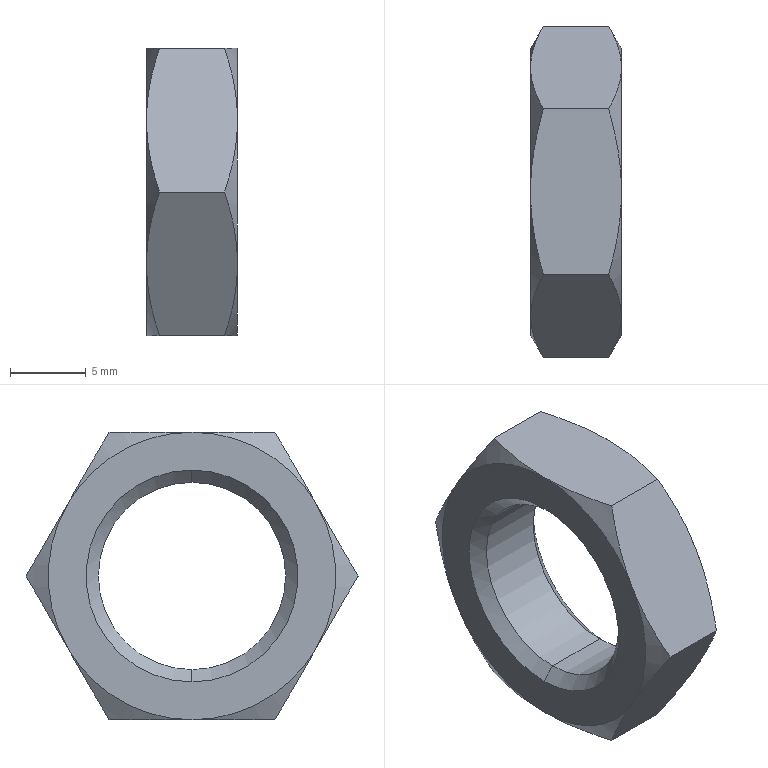Part | SolidWorks | features BaseBody 1 | 1 solid | 26 faces | box 6 x 21.939 x 19 mm | volume 1112 mm3 | cone 16 | plane 8 | cylinder 2 | commonest cylinder face diameters 12.376 x2
STEP:
#1=CARTESIAN_POINT('',(5.188,0.,-6.188));
#2=VERTEX_POINT('',#1);
#3=CARTESIAN_POINT('',(5.188,-6.188,0.));
#4=VERTEX_POINT('',#3);
#5=CARTESIAN_POINT('',(5.188,0.,0.));
#6=DIRECTION('',(-1.,0.,0.));
#7=DIRECTION('',(0.,0.,1.));
#8=AXIS2_PLACEMENT_3D('',#5,#6,#7);
#9=CIRCLE('',#8,6.188);
#10=EDGE_CURVE('',#2,#4,#9,.T.);
#11=ORIENTED_EDGE('',*,*,#10,.F.);
#12=CARTESIAN_POINT('',(0.812,0.,-6.188));
#13=VERTEX_POINT('',#12);
#14=CARTESIAN_POINT('',(50.,0.,-6.188));
#15=DIRECTION('',(-1.,0.,0.));
#16=VECTOR('',#15,1000.);
#17=LINE('',#14,#16);
#18=EDGE_CURVE('',#2,#13,#17,.T.);
#19=ORIENTED_EDGE('',*,*,#18,.T.);
#20=CARTESIAN_POINT('',(0.812,0.,6.188));
#21=VERTEX_POINT('',#20);
#22=CARTESIAN_POINT('',(0.812,0.,0.));
#23=DIRECTION('',(1.,0.,0.));
#24=DIRECTION('',(0.,0.,1.));
#25=AXIS2_PLACEMENT_3D('',#22,#23,#24);
#26=CIRCLE('',#25,6.188);
#27=EDGE_CURVE('',#21,#13,#26,.T.);
#28=ORIENTED_EDGE('',*,*,#27,.F.);
#29=CARTESIAN_POINT('',(5.188,0.,6.188));
#30=VERTEX_POINT('',#29);
#31=CARTESIAN_POINT('',(50.,0.,6.188));
#32=DIRECTION('',(-1.,0.,0.));
#33=VECTOR('',#32,1000.);
#34=LINE('',#31,#33);
#35=EDGE_CURVE('',#30,#21,#34,.T.);
#36=ORIENTED_EDGE('',*,*,#35,.F.);
#37=CARTESIAN_POINT('',(5.188,0.,0.));
#38=DIRECTION('',(-1.,0.,0.));
#39=DIRECTION('',(0.,0.,1.));
#40=AXIS2_PLACEMENT_3D('',#37,#38,#39);
#41=CIRCLE('',#40,6.188);
#42=EDGE_CURVE('',#4,#30,#41,.T.);
#43=ORIENTED_EDGE('',*,*,#42,.F.);
#44=EDGE_LOOP('',(#11,#19,#28,#36,#43));
#45=FACE_OUTER_BOUND('',#44,.T.);
#46=CARTESIAN_POINT('',(50.,0.,0.));
#47=DIRECTION('',(-1.,0.,0.));
#48=DIRECTION('',(0.,0.,1.));
#49=AXIS2_PLACEMENT_3D('',#46,#47,#48);
#50=CYLINDRICAL_SURFACE('',#49,6.188);
#51=ADVANCED_FACE('',(#45),#50,.F.);
#52=ORIENTED_EDGE('',*,*,#27,.T.);
#53=CARTESIAN_POINT('',(0.,0.,-7.));
#54=VERTEX_POINT('',#53);
#55=CARTESIAN_POINT('',(0.,0.,-7.));
#56=DIRECTION('',(-0.7071,0.,-0.7071));
#57=VECTOR('',#56,1000.);
#58=LINE('',#55,#57);
#59=EDGE_CURVE('',#13,#54,#58,.T.);
#60=ORIENTED_EDGE('',*,*,#59,.T.);
#61=CARTESIAN_POINT('',(0.,0.,7.));
#62=VERTEX_POINT('',#61);
#63=CARTESIAN_POINT('',(0.,0.,0.));
#64=DIRECTION('',(1.,0.,0.));
#65=DIRECTION('',(0.,0.,1.));
#66=AXIS2_PLACEMENT_3D('',#63,#64,#65);
#67=CIRCLE('',#66,7.);
#68=EDGE_CURVE('',#62,#54,#67,.T.);
#69=ORIENTED_EDGE('',*,*,#68,.F.);
#70=CARTESIAN_POINT('',(0.,0.,7.));
#71=DIRECTION('',(-0.7071,0.,0.7071));
#72=VECTOR('',#71,1000.);
#73=LINE('',#70,#72);
#74=EDGE_CURVE('',#21,#62,#73,.T.);
#75=ORIENTED_EDGE('',*,*,#74,.F.);
#76=EDGE_LOOP('',(#52,#60,#69,#75));
#77=FACE_OUTER_BOUND('',#76,.T.);
#78=CARTESIAN_POINT('',(0.,0.,0.));
#79=DIRECTION('',(-1.,0.,0.));
#80=DIRECTION('',(0.,0.,1.));
#81=AXIS2_PLACEMENT_3D('',#78,#79,#80);
#82=CONICAL_SURFACE('',#81,7.,0.7854);
#83=ADVANCED_FACE('',(#77),#82,.F.);
#84=CARTESIAN_POINT('',(5.188,6.188,0.));
#85=VERTEX_POINT('',#84);
#86=CARTESIAN_POINT('',(5.188,0.,0.));
#87=DIRECTION('',(-1.,0.,0.));
#88=DIRECTION('',(0.,0.,1.));
#89=AXIS2_PLACEMENT_3D('',#86,#87,#88);
#90=CIRCLE('',#89,6.188);
#91=EDGE_CURVE('',#85,#2,#90,.T.);
#92=ORIENTED_EDGE('',*,*,#91,.T.);
#93=ORIENTED_EDGE('',*,*,#10,.T.);
#94=CARTESIAN_POINT('',(6.,-7.,0.));
#95=VERTEX_POINT('',#94);
#96=CARTESIAN_POINT('',(6.,-7.,0.));
#97=DIRECTION('',(0.7071,-0.7071,0.));
#98=VECTOR('',#97,1000.);
#99=LINE('',#96,#98);
#100=EDGE_CURVE('',#4,#95,#99,.T.);
#101=ORIENTED_EDGE('',*,*,#100,.T.);
#102=CARTESIAN_POINT('',(6.,7.,0.));
#103=VERTEX_POINT('',#102);
#104=CARTESIAN_POINT('',(6.,0.,0.));
#105=DIRECTION('',(-1.,0.,0.));
#106=DIRECTION('',(0.,1.,0.));
#107=AXIS2_PLACEMENT_3D('',#104,#105,#106);
#108=CIRCLE('',#107,7.);
#109=EDGE_CURVE('',#103,#95,#108,.T.);
#110=ORIENTED_EDGE('',*,*,#109,.F.);
#111=CARTESIAN_POINT('',(6.,7.,0.));
#112=DIRECTION('',(0.7071,0.7071,0.));
#113=VECTOR('',#112,1000.);
#114=LINE('',#111,#113);
#115=EDGE_CURVE('',#85,#103,#114,.T.);
#116=ORIENTED_EDGE('',*,*,#115,.F.);
#117=EDGE_LOOP('',(#92,#93,#101,#110,#116));
#118=FACE_OUTER_BOUND('',#117,.T.);
#119=CARTESIAN_POINT('',(6.,0.,0.));
#120=DIRECTION('',(1.,0.,0.));
#121=DIRECTION('',(0.,1.,0.));
#122=AXIS2_PLACEMENT_3D('',#119,#120,#121);
#123=CONICAL_SURFACE('',#122,7.,0.7854);
#124=ADVANCED_FACE('',(#118),#123,.F.);
#125=ORIENTED_EDGE('',*,*,#18,.F.);
#126=ORIENTED_EDGE('',*,*,#91,.F.);
#127=CARTESIAN_POINT('',(5.188,0.,0.));
#128=DIRECTION('',(-1.,0.,0.));
#129=DIRECTION('',(0.,0.,1.));
#130=AXIS2_PLACEMENT_3D('',#127,#128,#129);
#131=CIRCLE('',#130,6.188);
#132=EDGE_CURVE('',#30,#85,#131,.T.);
#133=ORIENTED_EDGE('',*,*,#132,.F.);
#134=ORIENTED_EDGE('',*,*,#35,.T.);
#135=CARTESIAN_POINT('',(0.812,0.,0.));
#136=DIRECTION('',(1.,0.,0.));
#137=DIRECTION('',(0.,0.,1.));
#138=AXIS2_PLACEMENT_3D('',#135,#136,#137);
#139=CIRCLE('',#138,6.188);
#140=EDGE_CURVE('',#13,#21,#139,.T.);
#141=ORIENTED_EDGE('',*,*,#140,.F.);
#142=EDGE_LOOP('',(#125,#126,#133,#134,#141));
#143=FACE_OUTER_BOUND('',#142,.T.);
#144=CARTESIAN_POINT('',(50.,0.,0.));
#145=DIRECTION('',(-1.,0.,0.));
#146=DIRECTION('',(0.,0.,1.));
#147=AXIS2_PLACEMENT_3D('',#144,#145,#146);
#148=CYLINDRICAL_SURFACE('',#147,6.188);
#149=ADVANCED_FACE('',(#143),#148,.F.);
#150=ORIENTED_EDGE('',*,*,#59,.F.);
#151=ORIENTED_EDGE('',*,*,#140,.T.);
#152=ORIENTED_EDGE('',*,*,#74,.T.);
#153=CARTESIAN_POINT('',(0.,0.,0.));
#154=DIRECTION('',(1.,0.,0.));
#155=DIRECTION('',(0.,0.,1.));
#156=AXIS2_PLACEMENT_3D('',#153,#154,#155);
#157=CIRCLE('',#156,7.);
#158=EDGE_CURVE('',#54,#62,#157,.T.);
#159=ORIENTED_EDGE('',*,*,#158,.F.);
#160=EDGE_LOOP('',(#150,#151,#152,#159));
#161=FACE_OUTER_BOUND('',#160,.T.);
#162=CARTESIAN_POINT('',(0.,0.,0.));
#163=DIRECTION('',(-1.,0.,0.));
#164=DIRECTION('',(0.,0.,1.));
#165=AXIS2_PLACEMENT_3D('',#162,#163,#164);
#166=CONICAL_SURFACE('',#165,7.,0.7854);
#167=ADVANCED_FACE('',(#161),#166,.F.);
#168=ORIENTED_EDGE('',*,*,#100,.F.);
#169=ORIENTED_EDGE('',*,*,#42,.T.);
#170=ORIENTED_EDGE('',*,*,#132,.T.);
#171=ORIENTED_EDGE('',*,*,#115,.T.);
#172=CARTESIAN_POINT('',(6.,0.,0.));
#173=DIRECTION('',(-1.,0.,0.));
#174=DIRECTION('',(0.,1.,0.));
#175=AXIS2_PLACEMENT_3D('',#172,#173,#174);
#176=CIRCLE('',#175,7.);
#177=EDGE_CURVE('',#95,#103,#176,.T.);
#178=ORIENTED_EDGE('',*,*,#177,.F.);
#179=EDGE_LOOP('',(#168,#169,#170,#171,#178));
#180=FACE_OUTER_BOUND('',#179,.T.);
#181=CARTESIAN_POINT('',(6.,0.,0.));
#182=DIRECTION('',(1.,0.,0.));
#183=DIRECTION('',(0.,1.,0.));
#184=AXIS2_PLACEMENT_3D('',#181,#182,#183);
#185=CONICAL_SURFACE('',#184,7.,0.7854);
#186=ADVANCED_FACE('',(#180),#185,.F.);
#187=CARTESIAN_POINT('',(0.,-8.227,4.75));
#188=VERTEX_POINT('',#187);
#189=CARTESIAN_POINT('',(0.,0.,9.5));
#190=VERTEX_POINT('',#189);
#191=CARTESIAN_POINT('',(0.,0.,0.));
#192=DIRECTION('',(-1.,0.,0.));
#193=DIRECTION('',(0.,1.,0.));
#194=AXIS2_PLACEMENT_3D('',#191,#192,#193);
#195=CIRCLE('',#194,9.5);
#196=EDGE_CURVE('',#188,#190,#195,.T.);
#197=ORIENTED_EDGE('',*,*,#196,.T.);
#198=CARTESIAN_POINT('',(0.,8.227,4.75));
#199=VERTEX_POINT('',#198);
#200=CARTESIAN_POINT('',(0.,0.,0.));
#201=DIRECTION('',(-1.,0.,0.));
#202=DIRECTION('',(0.,1.,0.));
#203=AXIS2_PLACEMENT_3D('',#200,#201,#202);
#204=CIRCLE('',#203,9.5);
#205=EDGE_CURVE('',#190,#199,#204,.T.);
#206=ORIENTED_EDGE('',*,*,#205,.T.);
#207=CARTESIAN_POINT('',(0.,8.227,-4.75));
#208=VERTEX_POINT('',#207);
#209=CARTESIAN_POINT('',(0.,0.,0.));
#210=DIRECTION('',(-1.,0.,0.));
#211=DIRECTION('',(0.,0.,-1.));
#212=AXIS2_PLACEMENT_3D('',#209,#210,#211);
#213=CIRCLE('',#212,9.5);
#214=EDGE_CURVE('',#199,#208,#213,.T.);
#215=ORIENTED_EDGE('',*,*,#214,.T.);
#216=CARTESIAN_POINT('',(0.,0.,-9.5));
#217=VERTEX_POINT('',#216);
#218=CARTESIAN_POINT('',(0.,0.,0.));
#219=DIRECTION('',(-1.,0.,0.));
#220=DIRECTION('',(0.,1.,0.));
#221=AXIS2_PLACEMENT_3D('',#218,#219,#220);
#222=CIRCLE('',#221,9.5);
#223=EDGE_CURVE('',#208,#217,#222,.T.);
#224=ORIENTED_EDGE('',*,*,#223,.T.);
#225=CARTESIAN_POINT('',(0.,-8.227,-4.75));
#226=VERTEX_POINT('',#225);
#227=CARTESIAN_POINT('',(0.,0.,0.));
#228=DIRECTION('',(-1.,0.,0.));
#229=DIRECTION('',(0.,1.,0.));
#230=AXIS2_PLACEMENT_3D('',#227,#228,#229);
#231=CIRCLE('',#230,9.5);
#232=EDGE_CURVE('',#217,#226,#231,.T.);
#233=ORIENTED_EDGE('',*,*,#232,.T.);
#234=CARTESIAN_POINT('',(0.,0.,0.));
#235=DIRECTION('',(-1.,0.,0.));
#236=DIRECTION('',(0.,0.,-1.));
#237=AXIS2_PLACEMENT_3D('',#234,#235,#236);
#238=CIRCLE('',#237,9.5);
#239=EDGE_CURVE('',#226,#188,#238,.T.);
#240=ORIENTED_EDGE('',*,*,#239,.T.);
#241=EDGE_LOOP('',(#197,#206,#215,#224,#233,#240));
#242=FACE_OUTER_BOUND('',#241,.T.);
#243=ORIENTED_EDGE('',*,*,#68,.T.);
#244=ORIENTED_EDGE('',*,*,#158,.T.);
#245=EDGE_LOOP('',(#243,#244));
#246=FACE_BOUND('',#245,.T.);
#247=CARTESIAN_POINT('',(0.,9.5,0.));
#248=DIRECTION('',(-1.,0.,0.));
#249=DIRECTION('',(0.,0.,1.));
#250=AXIS2_PLACEMENT_3D('',#247,#248,#249);
#251=PLANE('',#250);
#252=ADVANCED_FACE('',(#242,#246),#251,.T.);
#253=ORIENTED_EDGE('',*,*,#109,.T.);
#254=ORIENTED_EDGE('',*,*,#177,.T.);
#255=EDGE_LOOP('',(#253,#254));
#256=FACE_BOUND('',#255,.T.);
#257=CARTESIAN_POINT('',(6.,-8.227,4.75));
#258=VERTEX_POINT('',#257);
#259=CARTESIAN_POINT('',(6.,-8.227,-4.75));
#260=VERTEX_POINT('',#259);
#261=CARTESIAN_POINT('',(6.,0.,0.));
#262=DIRECTION('',(1.,0.,0.));
#263=DIRECTION('',(0.,0.,1.));
#264=AXIS2_PLACEMENT_3D('',#261,#262,#263);
#265=CIRCLE('',#264,9.5);
#266=EDGE_CURVE('',#258,#260,#265,.T.);
#267=ORIENTED_EDGE('',*,*,#266,.T.);
#268=CARTESIAN_POINT('',(6.,0.,-9.5));
#269=VERTEX_POINT('',#268);
#270=CARTESIAN_POINT('',(6.,0.,0.));
#271=DIRECTION('',(1.,0.,0.));
#272=DIRECTION('',(0.,0.,1.));
#273=AXIS2_PLACEMENT_3D('',#270,#271,#272);
#274=CIRCLE('',#273,9.5);
#275=EDGE_CURVE('',#260,#269,#274,.T.);
#276=ORIENTED_EDGE('',*,*,#275,.T.);
#277=CARTESIAN_POINT('',(6.,8.227,-4.75));
#278=VERTEX_POINT('',#277);
#279=CARTESIAN_POINT('',(6.,0.,0.));
#280=DIRECTION('',(1.,0.,0.));
#281=DIRECTION('',(0.,0.,1.));
#282=AXIS2_PLACEMENT_3D('',#279,#280,#281);
#283=CIRCLE('',#282,9.5);
#284=EDGE_CURVE('',#269,#278,#283,.T.);
#285=ORIENTED_EDGE('',*,*,#284,.T.);
#286=CARTESIAN_POINT('',(6.,8.227,4.75));
#287=VERTEX_POINT('',#286);
#288=CARTESIAN_POINT('',(6.,0.,0.));
#289=DIRECTION('',(1.,0.,0.));
#290=DIRECTION('',(0.,0.,1.));
#291=AXIS2_PLACEMENT_3D('',#288,#289,#290);
#292=CIRCLE('',#291,9.5);
#293=EDGE_CURVE('',#278,#287,#292,.T.);
#294=ORIENTED_EDGE('',*,*,#293,.T.);
#295=CARTESIAN_POINT('',(6.,0.,9.5));
#296=VERTEX_POINT('',#295);
#297=CARTESIAN_POINT('',(6.,0.,0.));
#298=DIRECTION('',(1.,0.,0.));
#299=DIRECTION('',(0.,0.,1.));
#300=AXIS2_PLACEMENT_3D('',#297,#298,#299);
#301=CIRCLE('',#300,9.5);
#302=EDGE_CURVE('',#287,#296,#301,.T.);
#303=ORIENTED_EDGE('',*,*,#302,.T.);
#304=CARTESIAN_POINT('',(6.,0.,0.));
#305=DIRECTION('',(1.,0.,0.));
#306=DIRECTION('',(0.,0.,1.));
#307=AXIS2_PLACEMENT_3D('',#304,#305,#306);
#308=CIRCLE('',#307,9.5);
#309=EDGE_CURVE('',#296,#258,#308,.T.);
#310=ORIENTED_EDGE('',*,*,#309,.T.);
#311=EDGE_LOOP('',(#267,#276,#285,#294,#303,#310));
#312=FACE_OUTER_BOUND('',#311,.T.);
#313=CARTESIAN_POINT('',(6.,7.,0.));
#314=DIRECTION('',(1.,0.,0.));
#315=DIRECTION('',(0.,0.,-1.));
#316=AXIS2_PLACEMENT_3D('',#313,#314,#315);
#317=PLANE('',#316);
#318=ADVANCED_FACE('',(#256,#312),#317,.T.);
#319=ORIENTED_EDGE('',*,*,#205,.F.);
#320=CARTESIAN_POINT('',(0.8485,5.485,9.5));
#321=VERTEX_POINT('',#320);
#322=CARTESIAN_POINT('',(0.,0.,9.5));
#323=CARTESIAN_POINT('',(0.,0.936,9.5));
#324=CARTESIAN_POINT('',(0.08112,1.859,9.5));
#325=CARTESIAN_POINT('',(0.3765,3.686,9.5));
#326=CARTESIAN_POINT('',(0.5899,4.589,9.5));
#327=CARTESIAN_POINT('',(0.8485,5.485,9.5));
#328=B_SPLINE_CURVE_WITH_KNOTS('',3,(#322,#323,#324,#325,#326,#327),.UNSPECIFIED.,.F.,.F.,(4,2,4),(0.,0.002775,0.00555),.UNSPECIFIED.);
#329=EDGE_CURVE('',#190,#321,#328,.T.);
#330=ORIENTED_EDGE('',*,*,#329,.T.);
#331=CARTESIAN_POINT('',(0.8485,5.485,9.5));
#332=CARTESIAN_POINT('',(0.5899,5.933,8.724));
#333=CARTESIAN_POINT('',(0.3765,6.384,7.942));
#334=CARTESIAN_POINT('',(0.08112,7.298,6.36));
#335=CARTESIAN_POINT('',(0.,7.759,5.561));
#336=CARTESIAN_POINT('',(0.,8.227,4.75));
#337=B_SPLINE_CURVE_WITH_KNOTS('',3,(#331,#332,#333,#334,#335,#336),.UNSPECIFIED.,.F.,.F.,(4,2,4),(0.,0.002775,0.00555),.UNSPECIFIED.);
#338=EDGE_CURVE('',#321,#199,#337,.T.);
#339=ORIENTED_EDGE('',*,*,#338,.T.);
#340=EDGE_LOOP('',(#319,#330,#339));
#341=FACE_OUTER_BOUND('',#340,.T.);
#342=CARTESIAN_POINT('',(0.8536,0.,0.));
#343=DIRECTION('',(1.,0.,0.));
#344=DIRECTION('',(0.,1.,0.));
#345=AXIS2_PLACEMENT_3D('',#342,#343,#344);
#346=CONICAL_SURFACE('',#345,10.978,1.047);
#347=ADVANCED_FACE('',(#341),#346,.T.);
#348=ORIENTED_EDGE('',*,*,#196,.F.);
#349=CARTESIAN_POINT('',(0.8485,-5.485,9.5));
#350=VERTEX_POINT('',#349);
#351=CARTESIAN_POINT('',(0.,-8.227,4.75));
#352=CARTESIAN_POINT('',(0.,-7.759,5.561));
#353=CARTESIAN_POINT('',(0.08112,-7.298,6.36));
#354=CARTESIAN_POINT('',(0.3765,-6.384,7.942));
#355=CARTESIAN_POINT('',(0.5899,-5.933,8.724));
#356=CARTESIAN_POINT('',(0.8485,-5.485,9.5));
#357=B_SPLINE_CURVE_WITH_KNOTS('',3,(#351,#352,#353,#354,#355,#356),.UNSPECIFIED.,.F.,.F.,(4,2,4),(0.,0.002775,0.00555),.UNSPECIFIED.);
#358=EDGE_CURVE('',#188,#350,#357,.T.);
#359=ORIENTED_EDGE('',*,*,#358,.T.);
#360=CARTESIAN_POINT('',(0.8485,-5.485,9.5));
#361=CARTESIAN_POINT('',(0.5899,-4.589,9.5));
#362=CARTESIAN_POINT('',(0.3765,-3.686,9.5));
#363=CARTESIAN_POINT('',(0.08112,-1.859,9.5));
#364=CARTESIAN_POINT('',(0.,-0.936,9.5));
#365=CARTESIAN_POINT('',(0.,0.,9.5));
#366=B_SPLINE_CURVE_WITH_KNOTS('',3,(#360,#361,#362,#363,#364,#365),.UNSPECIFIED.,.F.,.F.,(4,2,4),(0.,0.002775,0.00555),.UNSPECIFIED.);
#367=EDGE_CURVE('',#350,#190,#366,.T.);
#368=ORIENTED_EDGE('',*,*,#367,.T.);
#369=EDGE_LOOP('',(#348,#359,#368));
#370=FACE_OUTER_BOUND('',#369,.T.);
#371=CARTESIAN_POINT('',(0.8536,0.,0.));
#372=DIRECTION('',(1.,0.,0.));
#373=DIRECTION('',(0.,1.,0.));
#374=AXIS2_PLACEMENT_3D('',#371,#372,#373);
#375=CONICAL_SURFACE('',#374,10.978,1.047);
#376=ADVANCED_FACE('',(#370),#375,.T.);
#377=CARTESIAN_POINT('',(0.8485,-10.97,-0.000000038));
#378=VERTEX_POINT('',#377);
#379=CARTESIAN_POINT('',(0.8485,-10.97,-0.000000038));
#380=CARTESIAN_POINT('',(0.5899,-10.522,0.776));
#381=CARTESIAN_POINT('',(0.3765,-10.07,1.558));
#382=CARTESIAN_POINT('',(0.08112,-9.157,3.14));
#383=CARTESIAN_POINT('',(0.,-8.695,3.939));
#384=CARTESIAN_POINT('',(0.,-8.227,4.75));
#385=B_SPLINE_CURVE_WITH_KNOTS('',3,(#379,#380,#381,#382,#383,#384),.UNSPECIFIED.,.F.,.F.,(4,2,4),(0.,0.002775,0.00555),.UNSPECIFIED.);
#386=EDGE_CURVE('',#378,#188,#385,.T.);
#387=ORIENTED_EDGE('',*,*,#386,.T.);
#388=ORIENTED_EDGE('',*,*,#239,.F.);
#389=CARTESIAN_POINT('',(0.,-8.227,-4.75));
#390=CARTESIAN_POINT('',(0.,-8.695,-3.939));
#391=CARTESIAN_POINT('',(0.08112,-9.157,-3.14));
#392=CARTESIAN_POINT('',(0.3765,-10.07,-1.558));
#393=CARTESIAN_POINT('',(0.5899,-10.522,-0.776));
#394=CARTESIAN_POINT('',(0.8485,-10.97,-0.000000038));
#395=B_SPLINE_CURVE_WITH_KNOTS('',3,(#389,#390,#391,#392,#393,#394),.UNSPECIFIED.,.F.,.F.,(4,2,4),(0.,0.002775,0.00555),.UNSPECIFIED.);
#396=EDGE_CURVE('',#226,#378,#395,.T.);
#397=ORIENTED_EDGE('',*,*,#396,.T.);
#398=EDGE_LOOP('',(#387,#388,#397));
#399=FACE_OUTER_BOUND('',#398,.T.);
#400=CARTESIAN_POINT('',(0.8536,0.,0.));
#401=DIRECTION('',(1.,0.,0.));
#402=DIRECTION('',(0.,0.,-1.));
#403=AXIS2_PLACEMENT_3D('',#400,#401,#402);
#404=CONICAL_SURFACE('',#403,10.978,1.047);
#405=ADVANCED_FACE('',(#399),#404,.T.);
#406=CARTESIAN_POINT('',(0.8485,-5.485,-9.5));
#407=VERTEX_POINT('',#406);
#408=CARTESIAN_POINT('',(0.8485,-5.485,-9.5));
#409=CARTESIAN_POINT('',(0.5899,-5.933,-8.724));
#410=CARTESIAN_POINT('',(0.3765,-6.384,-7.942));
#411=CARTESIAN_POINT('',(0.08112,-7.298,-6.36));
#412=CARTESIAN_POINT('',(0.,-7.759,-5.561));
#413=CARTESIAN_POINT('',(0.,-8.227,-4.75));
#414=B_SPLINE_CURVE_WITH_KNOTS('',3,(#408,#409,#410,#411,#412,#413),.UNSPECIFIED.,.F.,.F.,(4,2,4),(0.,0.002775,0.00555),.UNSPECIFIED.);
#415=EDGE_CURVE('',#407,#226,#414,.T.);
#416=ORIENTED_EDGE('',*,*,#415,.T.);
#417=ORIENTED_EDGE('',*,*,#232,.F.);
#418=CARTESIAN_POINT('',(0.,0.,-9.5));
#419=CARTESIAN_POINT('',(0.,-0.936,-9.5));
#420=CARTESIAN_POINT('',(0.08112,-1.859,-9.5));
#421=CARTESIAN_POINT('',(0.3765,-3.686,-9.5));
#422=CARTESIAN_POINT('',(0.5899,-4.589,-9.5));
#423=CARTESIAN_POINT('',(0.8485,-5.485,-9.5));
#424=B_SPLINE_CURVE_WITH_KNOTS('',3,(#418,#419,#420,#421,#422,#423),.UNSPECIFIED.,.F.,.F.,(4,2,4),(0.,0.002775,0.00555),.UNSPECIFIED.);
#425=EDGE_CURVE('',#217,#407,#424,.T.);
#426=ORIENTED_EDGE('',*,*,#425,.T.);
#427=EDGE_LOOP('',(#416,#417,#426));
#428=FACE_OUTER_BOUND('',#427,.T.);
#429=CARTESIAN_POINT('',(0.8536,0.,0.));
#430=DIRECTION('',(1.,0.,0.));
#431=DIRECTION('',(0.,1.,0.));
#432=AXIS2_PLACEMENT_3D('',#429,#430,#431);
#433=CONICAL_SURFACE('',#432,10.978,1.047);
#434=ADVANCED_FACE('',(#428),#433,.T.);
#435=CARTESIAN_POINT('',(0.8485,5.485,-9.5));
#436=VERTEX_POINT('',#435);
#437=CARTESIAN_POINT('',(0.8485,5.485,-9.5));
#438=CARTESIAN_POINT('',(0.5899,4.589,-9.5));
#439=CARTESIAN_POINT('',(0.3765,3.686,-9.5));
#440=CARTESIAN_POINT('',(0.08112,1.859,-9.5));
#441=CARTESIAN_POINT('',(0.,0.936,-9.5));
#442=CARTESIAN_POINT('',(0.,0.,-9.5));
#443=B_SPLINE_CURVE_WITH_KNOTS('',3,(#437,#438,#439,#440,#441,#442),.UNSPECIFIED.,.F.,.F.,(4,2,4),(0.,0.002775,0.00555),.UNSPECIFIED.);
#444=EDGE_CURVE('',#436,#217,#443,.T.);
#445=ORIENTED_EDGE('',*,*,#444,.T.);
#446=ORIENTED_EDGE('',*,*,#223,.F.);
#447=CARTESIAN_POINT('',(0.,8.227,-4.75));
#448=CARTESIAN_POINT('',(0.,7.759,-5.561));
#449=CARTESIAN_POINT('',(0.08112,7.298,-6.36));
#450=CARTESIAN_POINT('',(0.3765,6.384,-7.942));
#451=CARTESIAN_POINT('',(0.5899,5.933,-8.724));
#452=CARTESIAN_POINT('',(0.8485,5.485,-9.5));
#453=B_SPLINE_CURVE_WITH_KNOTS('',3,(#447,#448,#449,#450,#451,#452),.UNSPECIFIED.,.F.,.F.,(4,2,4),(0.,0.002775,0.00555),.UNSPECIFIED.);
#454=EDGE_CURVE('',#208,#436,#453,.T.);
#455=ORIENTED_EDGE('',*,*,#454,.T.);
#456=EDGE_LOOP('',(#445,#446,#455));
#457=FACE_OUTER_BOUND('',#456,.T.);
#458=CARTESIAN_POINT('',(0.8536,0.,0.));
#459=DIRECTION('',(1.,0.,0.));
#460=DIRECTION('',(0.,1.,0.));
#461=AXIS2_PLACEMENT_3D('',#458,#459,#460);
#462=CONICAL_SURFACE('',#461,10.978,1.047);
#463=ADVANCED_FACE('',(#457),#462,.T.);
#464=CARTESIAN_POINT('',(0.8485,10.97,0.000000038));
#465=VERTEX_POINT('',#464);
#466=CARTESIAN_POINT('',(0.8485,10.97,0.000000038));
#467=CARTESIAN_POINT('',(0.5899,10.522,-0.776));
#468=CARTESIAN_POINT('',(0.3765,10.07,-1.558));
#469=CARTESIAN_POINT('',(0.08112,9.157,-3.14));
#470=CARTESIAN_POINT('',(0.,8.695,-3.939));
#471=CARTESIAN_POINT('',(0.,8.227,-4.75));
#472=B_SPLINE_CURVE_WITH_KNOTS('',3,(#466,#467,#468,#469,#470,#471),.UNSPECIFIED.,.F.,.F.,(4,2,4),(0.,0.002775,0.00555),.UNSPECIFIED.);
#473=EDGE_CURVE('',#465,#208,#472,.T.);
#474=ORIENTED_EDGE('',*,*,#473,.T.);
#475=ORIENTED_EDGE('',*,*,#214,.F.);
#476=CARTESIAN_POINT('',(0.,8.227,4.75));
#477=CARTESIAN_POINT('',(0.,8.695,3.939));
#478=CARTESIAN_POINT('',(0.08112,9.157,3.14));
#479=CARTESIAN_POINT('',(0.3765,10.07,1.558));
#480=CARTESIAN_POINT('',(0.5899,10.522,0.776));
#481=CARTESIAN_POINT('',(0.8485,10.97,0.000000038));
#482=B_SPLINE_CURVE_WITH_KNOTS('',3,(#476,#477,#478,#479,#480,#481),.UNSPECIFIED.,.F.,.F.,(4,2,4),(0.,0.002775,0.00555),.UNSPECIFIED.);
#483=EDGE_CURVE('',#199,#465,#482,.T.);
#484=ORIENTED_EDGE('',*,*,#483,.T.);
#485=EDGE_LOOP('',(#474,#475,#484));
#486=FACE_OUTER_BOUND('',#485,.T.);
#487=CARTESIAN_POINT('',(0.8536,0.,0.));
#488=DIRECTION('',(1.,0.,0.));
#489=DIRECTION('',(0.,0.,-1.));
#490=AXIS2_PLACEMENT_3D('',#487,#488,#489);
#491=CONICAL_SURFACE('',#490,10.978,1.047);
#492=ADVANCED_FACE('',(#486),#491,.T.);
#493=ORIENTED_EDGE('',*,*,#275,.F.);
#494=CARTESIAN_POINT('',(5.151,-5.485,-9.5));
#495=VERTEX_POINT('',#494);
#496=CARTESIAN_POINT('',(6.,-8.227,-4.75));
#497=CARTESIAN_POINT('',(6.,-7.759,-5.561));
#498=CARTESIAN_POINT('',(5.919,-7.298,-6.36));
#499=CARTESIAN_POINT('',(5.623,-6.384,-7.942));
#500=CARTESIAN_POINT('',(5.41,-5.933,-8.724));
#501=CARTESIAN_POINT('',(5.151,-5.485,-9.5));
#502=B_SPLINE_CURVE_WITH_KNOTS('',3,(#496,#497,#498,#499,#500,#501),.UNSPECIFIED.,.F.,.F.,(4,2,4),(0.,0.002775,0.00555),.UNSPECIFIED.);
#503=EDGE_CURVE('',#260,#495,#502,.T.);
#504=ORIENTED_EDGE('',*,*,#503,.T.);
#505=CARTESIAN_POINT('',(5.151,-5.485,-9.5));
#506=CARTESIAN_POINT('',(5.41,-4.589,-9.5));
#507=CARTESIAN_POINT('',(5.623,-3.686,-9.5));
#508=CARTESIAN_POINT('',(5.919,-1.859,-9.5));
#509=CARTESIAN_POINT('',(6.,-0.936,-9.5));
#510=CARTESIAN_POINT('',(6.,0.,-9.5));
#511=B_SPLINE_CURVE_WITH_KNOTS('',3,(#505,#506,#507,#508,#509,#510),.UNSPECIFIED.,.F.,.F.,(4,2,4),(0.,0.002775,0.00555),.UNSPECIFIED.);
#512=EDGE_CURVE('',#495,#269,#511,.T.);
#513=ORIENTED_EDGE('',*,*,#512,.T.);
#514=EDGE_LOOP('',(#493,#504,#513));
#515=FACE_OUTER_BOUND('',#514,.T.);
#516=CARTESIAN_POINT('',(5.146,0.,0.));
#517=DIRECTION('',(-1.,0.,0.));
#518=DIRECTION('',(0.,0.,1.));
#519=AXIS2_PLACEMENT_3D('',#516,#517,#518);
#520=CONICAL_SURFACE('',#519,10.978,1.047);
#521=ADVANCED_FACE('',(#515),#520,.T.);
#522=ORIENTED_EDGE('',*,*,#266,.F.);
#523=CARTESIAN_POINT('',(5.151,-10.97,-0.000000014));
#524=VERTEX_POINT('',#523);
#525=CARTESIAN_POINT('',(6.,-8.227,4.75));
#526=CARTESIAN_POINT('',(6.,-8.695,3.939));
#527=CARTESIAN_POINT('',(5.919,-9.157,3.14));
#528=CARTESIAN_POINT('',(5.623,-10.07,1.558));
#529=CARTESIAN_POINT('',(5.41,-10.522,0.776));
#530=CARTESIAN_POINT('',(5.151,-10.97,-0.000000014));
#531=B_SPLINE_CURVE_WITH_KNOTS('',3,(#525,#526,#527,#528,#529,#530),.UNSPECIFIED.,.F.,.F.,(4,2,4),(0.,0.002775,0.00555),.UNSPECIFIED.);
#532=EDGE_CURVE('',#258,#524,#531,.T.);
#533=ORIENTED_EDGE('',*,*,#532,.T.);
#534=CARTESIAN_POINT('',(5.151,-10.97,-0.000000014));
#535=CARTESIAN_POINT('',(5.41,-10.522,-0.776));
#536=CARTESIAN_POINT('',(5.623,-10.07,-1.558));
#537=CARTESIAN_POINT('',(5.919,-9.157,-3.14));
#538=CARTESIAN_POINT('',(6.,-8.695,-3.939));
#539=CARTESIAN_POINT('',(6.,-8.227,-4.75));
#540=B_SPLINE_CURVE_WITH_KNOTS('',3,(#534,#535,#536,#537,#538,#539),.UNSPECIFIED.,.F.,.F.,(4,2,4),(0.,0.002775,0.00555),.UNSPECIFIED.);
#541=EDGE_CURVE('',#524,#260,#540,.T.);
#542=ORIENTED_EDGE('',*,*,#541,.T.);
#543=EDGE_LOOP('',(#522,#533,#542));
#544=FACE_OUTER_BOUND('',#543,.T.);
#545=CARTESIAN_POINT('',(5.146,0.,0.));
#546=DIRECTION('',(-1.,0.,0.));
#547=DIRECTION('',(0.,0.,1.));
#548=AXIS2_PLACEMENT_3D('',#545,#546,#547);
#549=CONICAL_SURFACE('',#548,10.978,1.047);
#550=ADVANCED_FACE('',(#544),#549,.T.);
#551=CARTESIAN_POINT('',(5.151,-5.485,9.5));
#552=VERTEX_POINT('',#551);
#553=CARTESIAN_POINT('',(5.151,-5.485,9.5));
#554=CARTESIAN_POINT('',(5.41,-5.933,8.724));
#555=CARTESIAN_POINT('',(5.623,-6.384,7.942));
#556=CARTESIAN_POINT('',(5.919,-7.298,6.36));
#557=CARTESIAN_POINT('',(6.,-7.759,5.561));
#558=CARTESIAN_POINT('',(6.,-8.227,4.75));
#559=B_SPLINE_CURVE_WITH_KNOTS('',3,(#553,#554,#555,#556,#557,#558),.UNSPECIFIED.,.F.,.F.,(4,2,4),(0.,0.002775,0.00555),.UNSPECIFIED.);
#560=EDGE_CURVE('',#552,#258,#559,.T.);
#561=ORIENTED_EDGE('',*,*,#560,.T.);
#562=ORIENTED_EDGE('',*,*,#309,.F.);
#563=CARTESIAN_POINT('',(6.,0.,9.5));
#564=CARTESIAN_POINT('',(6.,-0.936,9.5));
#565=CARTESIAN_POINT('',(5.919,-1.859,9.5));
#566=CARTESIAN_POINT('',(5.623,-3.686,9.5));
#567=CARTESIAN_POINT('',(5.41,-4.589,9.5));
#568=CARTESIAN_POINT('',(5.151,-5.485,9.5));
#569=B_SPLINE_CURVE_WITH_KNOTS('',3,(#563,#564,#565,#566,#567,#568),.UNSPECIFIED.,.F.,.F.,(4,2,4),(0.,0.002775,0.00555),.UNSPECIFIED.);
#570=EDGE_CURVE('',#296,#552,#569,.T.);
#571=ORIENTED_EDGE('',*,*,#570,.T.);
#572=EDGE_LOOP('',(#561,#562,#571));
#573=FACE_OUTER_BOUND('',#572,.T.);
#574=CARTESIAN_POINT('',(5.146,0.,0.));
#575=DIRECTION('',(-1.,0.,0.));
#576=DIRECTION('',(0.,0.,1.));
#577=AXIS2_PLACEMENT_3D('',#574,#575,#576);
#578=CONICAL_SURFACE('',#577,10.978,1.047);
#579=ADVANCED_FACE('',(#573),#578,.T.);
#580=ORIENTED_EDGE('',*,*,#302,.F.);
#581=CARTESIAN_POINT('',(5.151,5.485,9.5));
#582=VERTEX_POINT('',#581);
#583=CARTESIAN_POINT('',(6.,8.227,4.75));
#584=CARTESIAN_POINT('',(6.,7.759,5.561));
#585=CARTESIAN_POINT('',(5.919,7.298,6.36));
#586=CARTESIAN_POINT('',(5.623,6.384,7.942));
#587=CARTESIAN_POINT('',(5.41,5.933,8.724));
#588=CARTESIAN_POINT('',(5.151,5.485,9.5));
#589=B_SPLINE_CURVE_WITH_KNOTS('',3,(#583,#584,#585,#586,#587,#588),.UNSPECIFIED.,.F.,.F.,(4,2,4),(0.,0.002775,0.00555),.UNSPECIFIED.);
#590=EDGE_CURVE('',#287,#582,#589,.T.);
#591=ORIENTED_EDGE('',*,*,#590,.T.);
#592=CARTESIAN_POINT('',(5.151,5.485,9.5));
#593=CARTESIAN_POINT('',(5.41,4.589,9.5));
#594=CARTESIAN_POINT('',(5.623,3.686,9.5));
#595=CARTESIAN_POINT('',(5.919,1.859,9.5));
#596=CARTESIAN_POINT('',(6.,0.936,9.5));
#597=CARTESIAN_POINT('',(6.,0.,9.5));
#598=B_SPLINE_CURVE_WITH_KNOTS('',3,(#592,#593,#594,#595,#596,#597),.UNSPECIFIED.,.F.,.F.,(4,2,4),(0.,0.002775,0.00555),.UNSPECIFIED.);
#599=EDGE_CURVE('',#582,#296,#598,.T.);
#600=ORIENTED_EDGE('',*,*,#599,.T.);
#601=EDGE_LOOP('',(#580,#591,#600));
#602=FACE_OUTER_BOUND('',#601,.T.);
#603=CARTESIAN_POINT('',(5.146,0.,0.));
#604=DIRECTION('',(-1.,0.,0.));
#605=DIRECTION('',(0.,0.,1.));
#606=AXIS2_PLACEMENT_3D('',#603,#604,#605);
#607=CONICAL_SURFACE('',#606,10.978,1.047);
#608=ADVANCED_FACE('',(#602),#607,.T.);
#609=CARTESIAN_POINT('',(5.151,10.97,-0.000000038));
#610=VERTEX_POINT('',#609);
#611=CARTESIAN_POINT('',(5.151,10.97,-0.000000038));
#612=CARTESIAN_POINT('',(5.41,10.522,0.776));
#613=CARTESIAN_POINT('',(5.623,10.07,1.558));
#614=CARTESIAN_POINT('',(5.919,9.157,3.14));
#615=CARTESIAN_POINT('',(6.,8.695,3.939));
#616=CARTESIAN_POINT('',(6.,8.227,4.75));
#617=B_SPLINE_CURVE_WITH_KNOTS('',3,(#611,#612,#613,#614,#615,#616),.UNSPECIFIED.,.F.,.F.,(4,2,4),(0.,0.002775,0.00555),.UNSPECIFIED.);
#618=EDGE_CURVE('',#610,#287,#617,.T.);
#619=ORIENTED_EDGE('',*,*,#618,.T.);
#620=ORIENTED_EDGE('',*,*,#293,.F.);
#621=CARTESIAN_POINT('',(6.,8.227,-4.75));
#622=CARTESIAN_POINT('',(6.,8.695,-3.939));
#623=CARTESIAN_POINT('',(5.919,9.157,-3.14));
#624=CARTESIAN_POINT('',(5.623,10.07,-1.558));
#625=CARTESIAN_POINT('',(5.41,10.522,-0.776));
#626=CARTESIAN_POINT('',(5.151,10.97,-0.000000038));
#627=B_SPLINE_CURVE_WITH_KNOTS('',3,(#621,#622,#623,#624,#625,#626),.UNSPECIFIED.,.F.,.F.,(4,2,4),(0.,0.002775,0.00555),.UNSPECIFIED.);
#628=EDGE_CURVE('',#278,#610,#627,.T.);
#629=ORIENTED_EDGE('',*,*,#628,.T.);
#630=EDGE_LOOP('',(#619,#620,#629));
#631=FACE_OUTER_BOUND('',#630,.T.);
#632=CARTESIAN_POINT('',(5.146,0.,0.));
#633=DIRECTION('',(-1.,0.,0.));
#634=DIRECTION('',(0.,0.,1.));
#635=AXIS2_PLACEMENT_3D('',#632,#633,#634);
#636=CONICAL_SURFACE('',#635,10.978,1.047);
#637=ADVANCED_FACE('',(#631),#636,.T.);
#638=ORIENTED_EDGE('',*,*,#284,.F.);
#639=CARTESIAN_POINT('',(5.151,5.485,-9.5));
#640=VERTEX_POINT('',#639);
#641=CARTESIAN_POINT('',(6.,0.,-9.5));
#642=CARTESIAN_POINT('',(6.,0.936,-9.5));
#643=CARTESIAN_POINT('',(5.919,1.859,-9.5));
#644=CARTESIAN_POINT('',(5.623,3.686,-9.5));
#645=CARTESIAN_POINT('',(5.41,4.589,-9.5));
#646=CARTESIAN_POINT('',(5.151,5.485,-9.5));
#647=B_SPLINE_CURVE_WITH_KNOTS('',3,(#641,#642,#643,#644,#645,#646),.UNSPECIFIED.,.F.,.F.,(4,2,4),(0.,0.002775,0.00555),.UNSPECIFIED.);
#648=EDGE_CURVE('',#269,#640,#647,.T.);
#649=ORIENTED_EDGE('',*,*,#648,.T.);
#650=CARTESIAN_POINT('',(5.151,5.485,-9.5));
#651=CARTESIAN_POINT('',(5.41,5.933,-8.724));
#652=CARTESIAN_POINT('',(5.623,6.384,-7.942));
#653=CARTESIAN_POINT('',(5.919,7.298,-6.36));
#654=CARTESIAN_POINT('',(6.,7.759,-5.561));
#655=CARTESIAN_POINT('',(6.,8.227,-4.75));
#656=B_SPLINE_CURVE_WITH_KNOTS('',3,(#650,#651,#652,#653,#654,#655),.UNSPECIFIED.,.F.,.F.,(4,2,4),(0.,0.002775,0.00555),.UNSPECIFIED.);
#657=EDGE_CURVE('',#640,#278,#656,.T.);
#658=ORIENTED_EDGE('',*,*,#657,.T.);
#659=EDGE_LOOP('',(#638,#649,#658));
#660=FACE_OUTER_BOUND('',#659,.T.);
#661=CARTESIAN_POINT('',(5.146,0.,0.));
#662=DIRECTION('',(-1.,0.,0.));
#663=DIRECTION('',(0.,0.,1.));
#664=AXIS2_PLACEMENT_3D('',#661,#662,#663);
#665=CONICAL_SURFACE('',#664,10.978,1.047);
#666=ADVANCED_FACE('',(#660),#665,.T.);
#667=ORIENTED_EDGE('',*,*,#367,.F.);
#668=CARTESIAN_POINT('',(6.,-5.485,9.5));
#669=DIRECTION('',(-1.,0.,0.));
#670=VECTOR('',#669,1000.);
#671=LINE('',#668,#670);
#672=EDGE_CURVE('',#552,#350,#671,.T.);
#673=ORIENTED_EDGE('',*,*,#672,.F.);
#674=ORIENTED_EDGE('',*,*,#570,.F.);
#675=ORIENTED_EDGE('',*,*,#599,.F.);
#676=CARTESIAN_POINT('',(6.,5.485,9.5));
#677=DIRECTION('',(1.,0.,0.));
#678=VECTOR('',#677,1000.);
#679=LINE('',#676,#678);
#680=EDGE_CURVE('',#321,#582,#679,.T.);
#681=ORIENTED_EDGE('',*,*,#680,.F.);
#682=ORIENTED_EDGE('',*,*,#329,.F.);
#683=EDGE_LOOP('',(#667,#673,#674,#675,#681,#682));
#684=FACE_OUTER_BOUND('',#683,.T.);
#685=CARTESIAN_POINT('',(6.,5.485,9.5));
#686=DIRECTION('',(0.,0.,-1.));
#687=DIRECTION('',(-1.,0.,0.));
#688=AXIS2_PLACEMENT_3D('',#685,#686,#687);
#689=PLANE('',#688);
#690=ADVANCED_FACE('',(#684),#689,.F.);
#691=ORIENTED_EDGE('',*,*,#338,.F.);
#692=ORIENTED_EDGE('',*,*,#680,.T.);
#693=ORIENTED_EDGE('',*,*,#590,.F.);
#694=ORIENTED_EDGE('',*,*,#618,.F.);
#695=CARTESIAN_POINT('',(6.,10.97,0.));
#696=DIRECTION('',(1.,0.,0.));
#697=VECTOR('',#696,1000.);
#698=LINE('',#695,#697);
#699=EDGE_CURVE('',#465,#610,#698,.T.);
#700=ORIENTED_EDGE('',*,*,#699,.F.);
#701=ORIENTED_EDGE('',*,*,#483,.F.);
#702=EDGE_LOOP('',(#691,#692,#693,#694,#700,#701));
#703=FACE_OUTER_BOUND('',#702,.T.);
#704=CARTESIAN_POINT('',(6.,10.97,0.));
#705=DIRECTION('',(0.,-0.866,-0.5));
#706=DIRECTION('',(0.,0.5,-0.866));
#707=AXIS2_PLACEMENT_3D('',#704,#705,#706);
#708=PLANE('',#707);
#709=ADVANCED_FACE('',(#703),#708,.F.);
#710=ORIENTED_EDGE('',*,*,#386,.F.);
#711=CARTESIAN_POINT('',(6.,-10.97,0.));
#712=DIRECTION('',(-1.,0.,0.));
#713=VECTOR('',#712,1000.);
#714=LINE('',#711,#713);
#715=EDGE_CURVE('',#524,#378,#714,.T.);
#716=ORIENTED_EDGE('',*,*,#715,.F.);
#717=ORIENTED_EDGE('',*,*,#532,.F.);
#718=ORIENTED_EDGE('',*,*,#560,.F.);
#719=ORIENTED_EDGE('',*,*,#672,.T.);
#720=ORIENTED_EDGE('',*,*,#358,.F.);
#721=EDGE_LOOP('',(#710,#716,#717,#718,#719,#720));
#722=FACE_OUTER_BOUND('',#721,.T.);
#723=CARTESIAN_POINT('',(6.,-5.485,9.5));
#724=DIRECTION('',(0.,0.866,-0.5));
#725=DIRECTION('',(0.,0.5,0.866));
#726=AXIS2_PLACEMENT_3D('',#723,#724,#725);
#727=PLANE('',#726);
#728=ADVANCED_FACE('',(#722),#727,.F.);
#729=ORIENTED_EDGE('',*,*,#415,.F.);
#730=CARTESIAN_POINT('',(6.,-5.485,-9.5));
#731=DIRECTION('',(-1.,0.,0.));
#732=VECTOR('',#731,1000.);
#733=LINE('',#730,#732);
#734=EDGE_CURVE('',#495,#407,#733,.T.);
#735=ORIENTED_EDGE('',*,*,#734,.F.);
#736=ORIENTED_EDGE('',*,*,#503,.F.);
#737=ORIENTED_EDGE('',*,*,#541,.F.);
#738=ORIENTED_EDGE('',*,*,#715,.T.);
#739=ORIENTED_EDGE('',*,*,#396,.F.);
#740=EDGE_LOOP('',(#729,#735,#736,#737,#738,#739));
#741=FACE_OUTER_BOUND('',#740,.T.);
#742=CARTESIAN_POINT('',(6.,-10.97,0.));
#743=DIRECTION('',(0.,0.866,0.5));
#744=DIRECTION('',(0.,-0.5,0.866));
#745=AXIS2_PLACEMENT_3D('',#742,#743,#744);
#746=PLANE('',#745);
#747=ADVANCED_FACE('',(#741),#746,.F.);
#748=ORIENTED_EDGE('',*,*,#444,.F.);
#749=CARTESIAN_POINT('',(6.,5.485,-9.5));
#750=DIRECTION('',(-1.,0.,0.));
#751=VECTOR('',#750,1000.);
#752=LINE('',#749,#751);
#753=EDGE_CURVE('',#640,#436,#752,.T.);
#754=ORIENTED_EDGE('',*,*,#753,.F.);
#755=ORIENTED_EDGE('',*,*,#648,.F.);
#756=ORIENTED_EDGE('',*,*,#512,.F.);
#757=ORIENTED_EDGE('',*,*,#734,.T.);
#758=ORIENTED_EDGE('',*,*,#425,.F.);
#759=EDGE_LOOP('',(#748,#754,#755,#756,#757,#758));
#760=FACE_OUTER_BOUND('',#759,.T.);
#761=CARTESIAN_POINT('',(6.,-5.485,-9.5));
#762=DIRECTION('',(0.,0.,1.));
#763=DIRECTION('',(1.,0.,0.));
#764=AXIS2_PLACEMENT_3D('',#761,#762,#763);
#765=PLANE('',#764);
#766=ADVANCED_FACE('',(#760),#765,.F.);
#767=ORIENTED_EDGE('',*,*,#473,.F.);
#768=ORIENTED_EDGE('',*,*,#699,.T.);
#769=ORIENTED_EDGE('',*,*,#628,.F.);
#770=ORIENTED_EDGE('',*,*,#657,.F.);
#771=ORIENTED_EDGE('',*,*,#753,.T.);
#772=ORIENTED_EDGE('',*,*,#454,.F.);
#773=EDGE_LOOP('',(#767,#768,#769,#770,#771,#772));
#774=FACE_OUTER_BOUND('',#773,.T.);
#775=CARTESIAN_POINT('',(6.,5.485,-9.5));
#776=DIRECTION('',(0.,-0.866,0.5));
#777=DIRECTION('',(0.,-0.5,-0.866));
#778=AXIS2_PLACEMENT_3D('',#775,#776,#777);
#779=PLANE('',#778);
#780=ADVANCED_FACE('',(#774),#779,.F.);
#781=CLOSED_SHELL('',(#51,#83,#124,#149,#167,#186,#252,#318,#347,#376,#405,#434,#463,#492,#521,#550,#579,#608,#637,#666,#690,#709,#728,#747,#766,#780));
#782=MANIFOLD_SOLID_BREP('',#781);
#783=CARTESIAN_POINT('',(0.,0.,0.));
#784=DIRECTION('',(0.,0.,1.));
#785=DIRECTION('',(1.,0.,0.));
#786=AXIS2_PLACEMENT_3D('',#783,#784,#785);
#787=(LENGTH_UNIT()NAMED_UNIT(*)SI_UNIT(.MILLI.,.METRE.));
#788=UNCERTAINTY_MEASURE_WITH_UNIT(LENGTH_MEASURE(0.00001),#787,'','');
#789=(NAMED_UNIT(*)PLANE_ANGLE_UNIT()SI_UNIT($,.RADIAN.));
#790=(NAMED_UNIT(*)SI_UNIT($,.STERADIAN.)SOLID_ANGLE_UNIT());
#791=(GEOMETRIC_REPRESENTATION_CONTEXT(3)GLOBAL_UNCERTAINTY_ASSIGNED_CONTEXT((#788))GLOBAL_UNIT_ASSIGNED_CONTEXT((#787,#789,#790))REPRESENTATION_CONTEXT('',''));
#792=ADVANCED_BREP_SHAPE_REPRESENTATION('',(#782,#786),#791);